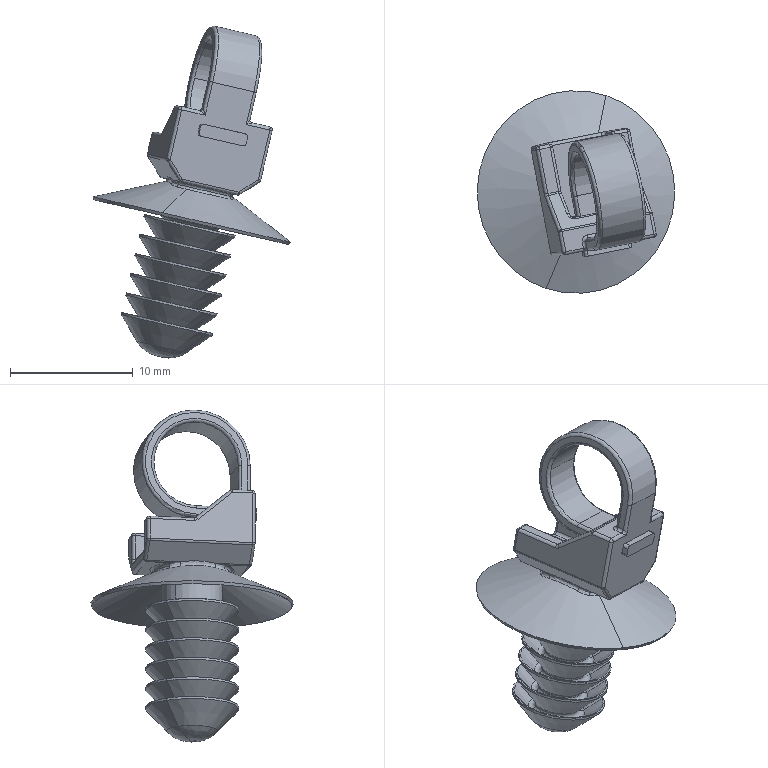Part | SolidWorks | features BaseBody 1 | 1 solid | 228 faces | box 16.092 x 16.511 x 27.057 mm | volume 643.939 mm3 | cylinder 79 | torus 46 | plane 33 | cone 32 | sphere 20 | spline 18 | commonest cylinder face diameters 0.5 x61 7.62 x10 4.92 x2 7 x2 7.619 x2 9 x2